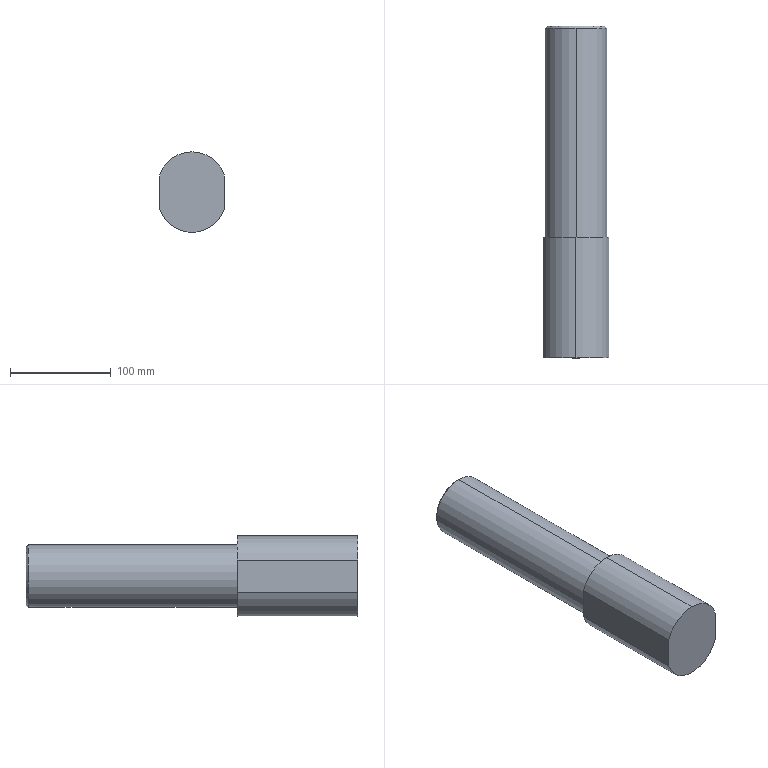Part | SolidWorks | features MirrorStock 1 | 1 solid | 16 faces | box 65 x 330 x 80 mm | volume 1156605 mm3 | cylinder 7 | plane 5 | cone 4 | commonest cylinder face diameters 68 x3 8.5 x2 62 x2
STEP:
#1=CARTESIAN_POINT('',(0.,330.,29.));
#2=VERTEX_POINT('',#1);
#3=CARTESIAN_POINT('',(0.,330.,-29.));
#4=VERTEX_POINT('',#3);
#5=CARTESIAN_POINT('',(0.,330.,0.));
#6=DIRECTION('',(0.,-1.,0.));
#7=DIRECTION('',(0.,0.,-1.));
#8=AXIS2_PLACEMENT_3D('',#5,#6,#7);
#9=CIRCLE('',#8,29.);
#10=EDGE_CURVE('',#2,#4,#9,.T.);
#11=ORIENTED_EDGE('',*,*,#10,.T.);
#12=CARTESIAN_POINT('',(0.,328.,-31.));
#13=VERTEX_POINT('',#12);
#14=CARTESIAN_POINT('',(0.,330.,-29.));
#15=DIRECTION('',(0.,-0.7071,-0.7071));
#16=VECTOR('',#15,1000.);
#17=LINE('',#14,#16);
#18=EDGE_CURVE('',#4,#13,#17,.T.);
#19=ORIENTED_EDGE('',*,*,#18,.T.);
#20=CARTESIAN_POINT('',(0.,328.,31.));
#21=VERTEX_POINT('',#20);
#22=CARTESIAN_POINT('',(0.,328.,0.));
#23=DIRECTION('',(0.,1.,0.));
#24=DIRECTION('',(0.,0.,-1.));
#25=AXIS2_PLACEMENT_3D('',#22,#23,#24);
#26=CIRCLE('',#25,31.);
#27=EDGE_CURVE('',#13,#21,#26,.T.);
#28=ORIENTED_EDGE('',*,*,#27,.T.);
#29=CARTESIAN_POINT('',(0.,330.,29.));
#30=DIRECTION('',(0.,-0.7071,0.7071));
#31=VECTOR('',#30,1000.);
#32=LINE('',#29,#31);
#33=EDGE_CURVE('',#2,#21,#32,.T.);
#34=ORIENTED_EDGE('',*,*,#33,.F.);
#35=EDGE_LOOP('',(#11,#19,#28,#34));
#36=FACE_OUTER_BOUND('',#35,.T.);
#37=CARTESIAN_POINT('',(0.,330.,0.));
#38=DIRECTION('',(0.,-1.,0.));
#39=DIRECTION('',(0.,0.,1.));
#40=AXIS2_PLACEMENT_3D('',#37,#38,#39);
#41=CONICAL_SURFACE('',#40,29.,0.7854);
#42=ADVANCED_FACE('',(#36),#41,.T.);
#43=CARTESIAN_POINT('',(0.,285.,-0.9463));
#44=VERTEX_POINT('',#43);
#45=CARTESIAN_POINT('',(4.25,285.,-3.5));
#46=VERTEX_POINT('',#45);
#47=CARTESIAN_POINT('',(4.25,285.,-3.5));
#48=DIRECTION('',(0.8572,0.,-0.515));
#49=VECTOR('',#48,1000.);
#50=LINE('',#47,#49);
#51=EDGE_CURVE('',#44,#46,#50,.T.);
#52=ORIENTED_EDGE('',*,*,#51,.F.);
#53=CARTESIAN_POINT('',(-4.25,285.,-3.5));
#54=VERTEX_POINT('',#53);
#55=CARTESIAN_POINT('',(-4.25,285.,-3.5));
#56=DIRECTION('',(-0.8572,0.,-0.515));
#57=VECTOR('',#56,1000.);
#58=LINE('',#55,#57);
#59=EDGE_CURVE('',#44,#54,#58,.T.);
#60=ORIENTED_EDGE('',*,*,#59,.T.);
#61=CARTESIAN_POINT('',(0.,285.,-3.5));
#62=DIRECTION('',(0.,0.,1.));
#63=DIRECTION('',(1.,0.,0.));
#64=AXIS2_PLACEMENT_3D('',#61,#62,#63);
#65=CIRCLE('',#64,4.25);
#66=EDGE_CURVE('',#46,#54,#65,.T.);
#67=ORIENTED_EDGE('',*,*,#66,.F.);
#68=EDGE_LOOP('',(#52,#60,#67));
#69=FACE_OUTER_BOUND('',#68,.T.);
#70=CARTESIAN_POINT('',(0.,285.,-3.5));
#71=DIRECTION('',(0.,0.,-1.));
#72=DIRECTION('',(1.,0.,0.));
#73=AXIS2_PLACEMENT_3D('',#70,#71,#72);
#74=CONICAL_SURFACE('',#73,4.25,1.03);
#75=ADVANCED_FACE('',(#69),#74,.F.);
#76=ORIENTED_EDGE('',*,*,#66,.T.);
#77=CARTESIAN_POINT('',(-4.25,285.,-30.707));
#78=VERTEX_POINT('',#77);
#79=CARTESIAN_POINT('',(-4.25,285.,-31.));
#80=DIRECTION('',(0.,0.,-1.));
#81=VECTOR('',#80,1000.);
#82=LINE('',#79,#81);
#83=EDGE_CURVE('',#54,#78,#82,.T.);
#84=ORIENTED_EDGE('',*,*,#83,.T.);
#85=CARTESIAN_POINT('',(0.,289.25,-31.));
#86=VERTEX_POINT('',#85);
#87=CARTESIAN_POINT('',(-4.25,285.,-30.707));
#88=CARTESIAN_POINT('',(-4.25,285.278,-30.707));
#89=CARTESIAN_POINT('',(-4.223,285.554,-30.711));
#90=CARTESIAN_POINT('',(-4.114,286.103,-30.726));
#91=CARTESIAN_POINT('',(-4.032,286.371,-30.737));
#92=CARTESIAN_POINT('',(-3.82,286.883,-30.764));
#93=CARTESIAN_POINT('',(-3.688,287.13,-30.78));
#94=CARTESIAN_POINT('',(-3.378,287.594,-30.816));
#95=CARTESIAN_POINT('',(-3.202,287.808,-30.835));
#96=CARTESIAN_POINT('',(-2.81,288.2,-30.873));
#97=CARTESIAN_POINT('',(-2.592,288.38,-30.892));
#98=CARTESIAN_POINT('',(-2.13,288.688,-30.928));
#99=CARTESIAN_POINT('',(-1.886,288.819,-30.944));
#100=CARTESIAN_POINT('',(-1.371,289.032,-30.971));
#101=CARTESIAN_POINT('',(-1.102,289.114,-30.982));
#102=CARTESIAN_POINT('',(-0.5579,289.222,-30.996));
#103=CARTESIAN_POINT('',(-0.281,289.25,-31.));
#104=CARTESIAN_POINT('',(0.,289.25,-31.));
#105=B_SPLINE_CURVE_WITH_KNOTS('',3,(#87,#88,#89,#90,#91,#92,#93,#94,#95,#96,#97,#98,#99,#100,#101,#102,#103,#104),.UNSPECIFIED.,.F.,.F.,(4,2,2,2,2,2,2,2,4),(0.0133,0.01413,0.01497,0.0158,0.01663,0.01746,0.01829,0.01912,0.01996),.UNSPECIFIED.);
#106=EDGE_CURVE('',#78,#86,#105,.T.);
#107=ORIENTED_EDGE('',*,*,#106,.T.);
#108=CARTESIAN_POINT('',(4.25,285.,-30.707));
#109=VERTEX_POINT('',#108);
#110=CARTESIAN_POINT('',(0.,289.25,-31.));
#111=CARTESIAN_POINT('',(0.2808,289.25,-31.));
#112=CARTESIAN_POINT('',(0.5569,289.222,-30.996));
#113=CARTESIAN_POINT('',(1.1,289.114,-30.982));
#114=CARTESIAN_POINT('',(1.371,289.033,-30.971));
#115=CARTESIAN_POINT('',(1.885,288.819,-30.944));
#116=CARTESIAN_POINT('',(2.128,288.689,-30.928));
#117=CARTESIAN_POINT('',(2.59,288.381,-30.892));
#118=CARTESIAN_POINT('',(2.808,288.202,-30.873));
#119=CARTESIAN_POINT('',(3.2,287.811,-30.835));
#120=CARTESIAN_POINT('',(3.376,287.597,-30.816));
#121=CARTESIAN_POINT('',(3.687,287.133,-30.78));
#122=CARTESIAN_POINT('',(3.818,286.886,-30.764));
#123=CARTESIAN_POINT('',(4.031,286.376,-30.737));
#124=CARTESIAN_POINT('',(4.113,286.108,-30.726));
#125=CARTESIAN_POINT('',(4.222,285.559,-30.711));
#126=CARTESIAN_POINT('',(4.25,285.281,-30.707));
#127=CARTESIAN_POINT('',(4.25,285.,-30.707));
#128=B_SPLINE_CURVE_WITH_KNOTS('',3,(#110,#111,#112,#113,#114,#115,#116,#117,#118,#119,#120,#121,#122,#123,#124,#125,#126,#127),.UNSPECIFIED.,.F.,.F.,(4,2,2,2,2,2,2,2,4),(0.01996,0.02079,0.02162,0.02245,0.02328,0.02411,0.02494,0.02577,0.0266),.UNSPECIFIED.);
#129=EDGE_CURVE('',#86,#109,#128,.T.);
#130=ORIENTED_EDGE('',*,*,#129,.T.);
#131=CARTESIAN_POINT('',(4.25,285.,-31.));
#132=DIRECTION('',(0.,0.,-1.));
#133=VECTOR('',#132,1000.);
#134=LINE('',#131,#133);
#135=EDGE_CURVE('',#46,#109,#134,.T.);
#136=ORIENTED_EDGE('',*,*,#135,.F.);
#137=EDGE_LOOP('',(#76,#84,#107,#130,#136));
#138=FACE_OUTER_BOUND('',#137,.T.);
#139=CARTESIAN_POINT('',(0.,285.,-31.));
#140=DIRECTION('',(0.,0.,-1.));
#141=DIRECTION('',(1.,0.,0.));
#142=AXIS2_PLACEMENT_3D('',#139,#140,#141);
#143=CYLINDRICAL_SURFACE('',#142,4.25);
#144=ADVANCED_FACE('',(#138),#143,.F.);
#145=ORIENTED_EDGE('',*,*,#27,.F.);
#146=CARTESIAN_POINT('',(0.,330.,-31.));
#147=DIRECTION('',(0.,-1.,0.));
#148=VECTOR('',#147,1000.);
#149=LINE('',#146,#148);
#150=EDGE_CURVE('',#13,#86,#149,.T.);
#151=ORIENTED_EDGE('',*,*,#150,.T.);
#152=ORIENTED_EDGE('',*,*,#106,.F.);
#153=CARTESIAN_POINT('',(0.,280.75,-31.));
#154=VERTEX_POINT('',#153);
#155=CARTESIAN_POINT('',(0.,280.75,-31.));
#156=CARTESIAN_POINT('',(-0.2775,280.75,-31.));
#157=CARTESIAN_POINT('',(-0.5594,280.778,-30.996));
#158=CARTESIAN_POINT('',(-1.105,280.887,-30.982));
#159=CARTESIAN_POINT('',(-1.37,280.967,-30.971));
#160=CARTESIAN_POINT('',(-1.884,281.18,-30.944));
#161=CARTESIAN_POINT('',(-2.133,281.313,-30.927));
#162=CARTESIAN_POINT('',(-2.593,281.621,-30.892));
#163=CARTESIAN_POINT('',(-2.807,281.797,-30.873));
#164=CARTESIAN_POINT('',(-3.204,282.193,-30.835));
#165=CARTESIAN_POINT('',(-3.379,282.408,-30.816));
#166=CARTESIAN_POINT('',(-3.687,282.868,-30.78));
#167=CARTESIAN_POINT('',(-3.82,283.116,-30.764));
#168=CARTESIAN_POINT('',(-4.033,283.631,-30.737));
#169=CARTESIAN_POINT('',(-4.113,283.895,-30.726));
#170=CARTESIAN_POINT('',(-4.222,284.441,-30.711));
#171=CARTESIAN_POINT('',(-4.25,284.723,-30.707));
#172=CARTESIAN_POINT('',(-4.25,285.,-30.707));
#173=B_SPLINE_CURVE_WITH_KNOTS('',3,(#155,#156,#157,#158,#159,#160,#161,#162,#163,#164,#165,#166,#167,#168,#169,#170,#171,#172),.UNSPECIFIED.,.F.,.F.,(4,2,2,2,2,2,2,2,4),(0.006653,0.007484,0.008316,0.009147,0.009978,0.01081,0.01164,0.01247,0.0133),.UNSPECIFIED.);
#174=EDGE_CURVE('',#154,#78,#173,.T.);
#175=ORIENTED_EDGE('',*,*,#174,.F.);
#176=CARTESIAN_POINT('',(0.,120.,-31.));
#177=VERTEX_POINT('',#176);
#178=CARTESIAN_POINT('',(0.,330.,-31.));
#179=DIRECTION('',(0.,-1.,0.));
#180=VECTOR('',#179,1000.);
#181=LINE('',#178,#180);
#182=EDGE_CURVE('',#154,#177,#181,.T.);
#183=ORIENTED_EDGE('',*,*,#182,.T.);
#184=CARTESIAN_POINT('',(0.,120.,31.));
#185=VERTEX_POINT('',#184);
#186=CARTESIAN_POINT('',(0.,120.,0.));
#187=DIRECTION('',(0.,-1.,0.));
#188=DIRECTION('',(0.,0.,-1.));
#189=AXIS2_PLACEMENT_3D('',#186,#187,#188);
#190=CIRCLE('',#189,31.);
#191=EDGE_CURVE('',#185,#177,#190,.T.);
#192=ORIENTED_EDGE('',*,*,#191,.F.);
#193=CARTESIAN_POINT('',(0.,330.,31.));
#194=DIRECTION('',(0.,-1.,0.));
#195=VECTOR('',#194,1000.);
#196=LINE('',#193,#195);
#197=EDGE_CURVE('',#21,#185,#196,.T.);
#198=ORIENTED_EDGE('',*,*,#197,.F.);
#199=EDGE_LOOP('',(#145,#151,#152,#175,#183,#192,#198));
#200=FACE_OUTER_BOUND('',#199,.T.);
#201=CARTESIAN_POINT('',(0.,330.,0.));
#202=DIRECTION('',(0.,-1.,0.));
#203=DIRECTION('',(0.,0.,1.));
#204=AXIS2_PLACEMENT_3D('',#201,#202,#203);
#205=CYLINDRICAL_SURFACE('',#204,31.);
#206=ADVANCED_FACE('',(#200),#205,.T.);
#207=CARTESIAN_POINT('',(32.5,120.,15.987));
#208=VERTEX_POINT('',#207);
#209=CARTESIAN_POINT('',(0.,120.,40.));
#210=VERTEX_POINT('',#209);
#211=CARTESIAN_POINT('',(0.,120.,6.));
#212=DIRECTION('',(0.,-1.,0.));
#213=DIRECTION('',(0.,0.,-1.));
#214=AXIS2_PLACEMENT_3D('',#211,#212,#213);
#215=CIRCLE('',#214,34.);
#216=EDGE_CURVE('',#208,#210,#215,.T.);
#217=ORIENTED_EDGE('',*,*,#216,.T.);
#218=CARTESIAN_POINT('',(0.,0.,40.));
#219=VERTEX_POINT('',#218);
#220=CARTESIAN_POINT('',(0.,120.,40.));
#221=DIRECTION('',(0.,-1.,0.));
#222=VECTOR('',#221,1000.);
#223=LINE('',#220,#222);
#224=EDGE_CURVE('',#210,#219,#223,.T.);
#225=ORIENTED_EDGE('',*,*,#224,.T.);
#226=CARTESIAN_POINT('',(32.5,0.,15.987));
#227=VERTEX_POINT('',#226);
#228=CARTESIAN_POINT('',(0.,0.,6.));
#229=DIRECTION('',(0.,-1.,0.));
#230=DIRECTION('',(0.,0.,-1.));
#231=AXIS2_PLACEMENT_3D('',#228,#229,#230);
#232=CIRCLE('',#231,34.);
#233=EDGE_CURVE('',#227,#219,#232,.T.);
#234=ORIENTED_EDGE('',*,*,#233,.F.);
#235=CARTESIAN_POINT('',(32.5,120.,15.987));
#236=DIRECTION('',(0.,-1.,0.));
#237=VECTOR('',#236,1000.);
#238=LINE('',#235,#237);
#239=EDGE_CURVE('',#208,#227,#238,.T.);
#240=ORIENTED_EDGE('',*,*,#239,.F.);
#241=EDGE_LOOP('',(#217,#225,#234,#240));
#242=FACE_OUTER_BOUND('',#241,.T.);
#243=CARTESIAN_POINT('',(0.,120.,6.));
#244=DIRECTION('',(0.,-1.,0.));
#245=DIRECTION('',(0.,0.,1.));
#246=AXIS2_PLACEMENT_3D('',#243,#244,#245);
#247=CYLINDRICAL_SURFACE('',#246,34.);
#248=ADVANCED_FACE('',(#242),#247,.T.);
#249=ORIENTED_EDGE('',*,*,#224,.F.);
#250=CARTESIAN_POINT('',(-32.5,120.,15.987));
#251=VERTEX_POINT('',#250);
#252=CARTESIAN_POINT('',(0.,120.,6.));
#253=DIRECTION('',(0.,-1.,0.));
#254=DIRECTION('',(0.,0.,-1.));
#255=AXIS2_PLACEMENT_3D('',#252,#253,#254);
#256=CIRCLE('',#255,34.);
#257=EDGE_CURVE('',#210,#251,#256,.T.);
#258=ORIENTED_EDGE('',*,*,#257,.T.);
#259=CARTESIAN_POINT('',(-32.5,0.,15.987));
#260=VERTEX_POINT('',#259);
#261=CARTESIAN_POINT('',(-32.5,120.,15.987));
#262=DIRECTION('',(0.,-1.,0.));
#263=VECTOR('',#262,1000.);
#264=LINE('',#261,#263);
#265=EDGE_CURVE('',#251,#260,#264,.T.);
#266=ORIENTED_EDGE('',*,*,#265,.T.);
#267=CARTESIAN_POINT('',(0.,0.,6.));
#268=DIRECTION('',(0.,-1.,0.));
#269=DIRECTION('',(0.,0.,-1.));
#270=AXIS2_PLACEMENT_3D('',#267,#268,#269);
#271=CIRCLE('',#270,34.);
#272=EDGE_CURVE('',#219,#260,#271,.T.);
#273=ORIENTED_EDGE('',*,*,#272,.F.);
#274=EDGE_LOOP('',(#249,#258,#266,#273));
#275=FACE_OUTER_BOUND('',#274,.T.);
#276=CARTESIAN_POINT('',(0.,120.,6.));
#277=DIRECTION('',(0.,-1.,0.));
#278=DIRECTION('',(0.,0.,1.));
#279=AXIS2_PLACEMENT_3D('',#276,#277,#278);
#280=CYLINDRICAL_SURFACE('',#279,34.);
#281=ADVANCED_FACE('',(#275),#280,.T.);
#282=CARTESIAN_POINT('',(-32.5,0.,-15.987));
#283=VERTEX_POINT('',#282);
#284=CARTESIAN_POINT('',(-32.5,0.,-15.987));
#285=DIRECTION('',(0.,0.,-1.));
#286=VECTOR('',#285,1000.);
#287=LINE('',#284,#286);
#288=EDGE_CURVE('',#260,#283,#287,.T.);
#289=ORIENTED_EDGE('',*,*,#288,.F.);
#290=ORIENTED_EDGE('',*,*,#265,.F.);
#291=CARTESIAN_POINT('',(-32.5,120.,-15.987));
#292=VERTEX_POINT('',#291);
#293=CARTESIAN_POINT('',(-32.5,120.,-15.987));
#294=DIRECTION('',(0.,0.,-1.));
#295=VECTOR('',#294,1000.);
#296=LINE('',#293,#295);
#297=EDGE_CURVE('',#251,#292,#296,.T.);
#298=ORIENTED_EDGE('',*,*,#297,.T.);
#299=CARTESIAN_POINT('',(-32.5,120.,-15.987));
#300=DIRECTION('',(0.,-1.,0.));
#301=VECTOR('',#300,1000.);
#302=LINE('',#299,#301);
#303=EDGE_CURVE('',#292,#283,#302,.T.);
#304=ORIENTED_EDGE('',*,*,#303,.T.);
#305=EDGE_LOOP('',(#289,#290,#298,#304));
#306=FACE_OUTER_BOUND('',#305,.T.);
#307=CARTESIAN_POINT('',(-32.5,120.,-15.987));
#308=DIRECTION('',(1.,0.,0.));
#309=DIRECTION('',(0.,0.,1.));
#310=AXIS2_PLACEMENT_3D('',#307,#308,#309);
#311=PLANE('',#310);
#312=ADVANCED_FACE('',(#306),#311,.F.);
#313=CARTESIAN_POINT('',(32.5,0.,-15.987));
#314=VERTEX_POINT('',#313);
#315=CARTESIAN_POINT('',(0.,0.,-6.));
#316=DIRECTION('',(0.,-1.,0.));
#317=DIRECTION('',(0.,0.,1.));
#318=AXIS2_PLACEMENT_3D('',#315,#316,#317);
#319=CIRCLE('',#318,34.);
#320=EDGE_CURVE('',#283,#314,#319,.T.);
#321=ORIENTED_EDGE('',*,*,#320,.F.);
#322=ORIENTED_EDGE('',*,*,#303,.F.);
#323=CARTESIAN_POINT('',(32.5,120.,-15.987));
#324=VERTEX_POINT('',#323);
#325=CARTESIAN_POINT('',(0.,120.,-6.));
#326=DIRECTION('',(0.,-1.,0.));
#327=DIRECTION('',(0.,0.,1.));
#328=AXIS2_PLACEMENT_3D('',#325,#326,#327);
#329=CIRCLE('',#328,34.);
#330=EDGE_CURVE('',#292,#324,#329,.T.);
#331=ORIENTED_EDGE('',*,*,#330,.T.);
#332=CARTESIAN_POINT('',(32.5,120.,-15.987));
#333=DIRECTION('',(0.,-1.,0.));
#334=VECTOR('',#333,1000.);
#335=LINE('',#332,#334);
#336=EDGE_CURVE('',#324,#314,#335,.T.);
#337=ORIENTED_EDGE('',*,*,#336,.T.);
#338=EDGE_LOOP('',(#321,#322,#331,#337));
#339=FACE_OUTER_BOUND('',#338,.T.);
#340=CARTESIAN_POINT('',(0.,120.,-6.));
#341=DIRECTION('',(0.,-1.,0.));
#342=DIRECTION('',(0.,0.,1.));
#343=AXIS2_PLACEMENT_3D('',#340,#341,#342);
#344=CYLINDRICAL_SURFACE('',#343,34.);
#345=ADVANCED_FACE('',(#339),#344,.T.);
#346=CARTESIAN_POINT('',(32.5,0.,-15.987));
#347=DIRECTION('',(0.,0.,1.));
#348=VECTOR('',#347,1000.);
#349=LINE('',#346,#348);
#350=EDGE_CURVE('',#314,#227,#349,.T.);
#351=ORIENTED_EDGE('',*,*,#350,.F.);
#352=ORIENTED_EDGE('',*,*,#336,.F.);
#353=CARTESIAN_POINT('',(32.5,120.,-15.987));
#354=DIRECTION('',(0.,0.,1.));
#355=VECTOR('',#354,1000.);
#356=LINE('',#353,#355);
#357=EDGE_CURVE('',#324,#208,#356,.T.);
#358=ORIENTED_EDGE('',*,*,#357,.T.);
#359=ORIENTED_EDGE('',*,*,#239,.T.);
#360=EDGE_LOOP('',(#351,#352,#358,#359));
#361=FACE_OUTER_BOUND('',#360,.T.);
#362=CARTESIAN_POINT('',(32.5,120.,-15.987));
#363=DIRECTION('',(-1.,0.,0.));
#364=DIRECTION('',(0.,0.,-1.));
#365=AXIS2_PLACEMENT_3D('',#362,#363,#364);
#366=PLANE('',#365);
#367=ADVANCED_FACE('',(#361),#366,.F.);
#368=ORIENTED_EDGE('',*,*,#191,.T.);
#369=CARTESIAN_POINT('',(0.,120.,0.));
#370=DIRECTION('',(0.,-1.,0.));
#371=DIRECTION('',(0.,0.,-1.));
#372=AXIS2_PLACEMENT_3D('',#369,#370,#371);
#373=CIRCLE('',#372,31.);
#374=EDGE_CURVE('',#177,#185,#373,.T.);
#375=ORIENTED_EDGE('',*,*,#374,.T.);
#376=EDGE_LOOP('',(#368,#375));
#377=FACE_BOUND('',#376,.T.);
#378=ORIENTED_EDGE('',*,*,#216,.F.);
#379=ORIENTED_EDGE('',*,*,#357,.F.);
#380=ORIENTED_EDGE('',*,*,#330,.F.);
#381=ORIENTED_EDGE('',*,*,#297,.F.);
#382=ORIENTED_EDGE('',*,*,#257,.F.);
#383=EDGE_LOOP('',(#378,#379,#380,#381,#382));
#384=FACE_OUTER_BOUND('',#383,.T.);
#385=CARTESIAN_POINT('',(0.,120.,6.));
#386=DIRECTION('',(0.,1.,0.));
#387=DIRECTION('',(0.,0.,-1.));
#388=AXIS2_PLACEMENT_3D('',#385,#386,#387);
#389=PLANE('',#388);
#390=ADVANCED_FACE('',(#377,#384),#389,.T.);
#391=ORIENTED_EDGE('',*,*,#233,.T.);
#392=ORIENTED_EDGE('',*,*,#272,.T.);
#393=ORIENTED_EDGE('',*,*,#288,.T.);
#394=ORIENTED_EDGE('',*,*,#320,.T.);
#395=ORIENTED_EDGE('',*,*,#350,.T.);
#396=EDGE_LOOP('',(#391,#392,#393,#394,#395));
#397=FACE_OUTER_BOUND('',#396,.T.);
#398=CARTESIAN_POINT('',(0.,0.,6.));
#399=DIRECTION('',(0.,1.,0.));
#400=DIRECTION('',(0.,0.,-1.));
#401=AXIS2_PLACEMENT_3D('',#398,#399,#400);
#402=PLANE('',#401);
#403=ADVANCED_FACE('',(#397),#402,.F.);
#404=ORIENTED_EDGE('',*,*,#150,.F.);
#405=CARTESIAN_POINT('',(0.,328.,0.));
#406=DIRECTION('',(0.,1.,0.));
#407=DIRECTION('',(0.,0.,-1.));
#408=AXIS2_PLACEMENT_3D('',#405,#406,#407);
#409=CIRCLE('',#408,31.);
#410=EDGE_CURVE('',#21,#13,#409,.T.);
#411=ORIENTED_EDGE('',*,*,#410,.F.);
#412=ORIENTED_EDGE('',*,*,#197,.T.);
#413=ORIENTED_EDGE('',*,*,#374,.F.);
#414=ORIENTED_EDGE('',*,*,#182,.F.);
#415=CARTESIAN_POINT('',(4.25,285.,-30.707));
#416=CARTESIAN_POINT('',(4.25,284.719,-30.707));
#417=CARTESIAN_POINT('',(4.222,284.442,-30.711));
#418=CARTESIAN_POINT('',(4.114,283.899,-30.726));
#419=CARTESIAN_POINT('',(4.032,283.628,-30.737));
#420=CARTESIAN_POINT('',(3.819,283.114,-30.764));
#421=CARTESIAN_POINT('',(3.688,282.87,-30.78));
#422=CARTESIAN_POINT('',(3.379,282.408,-30.816));
#423=CARTESIAN_POINT('',(3.2,282.189,-30.835));
#424=CARTESIAN_POINT('',(2.808,281.798,-30.873));
#425=CARTESIAN_POINT('',(2.594,281.622,-30.892));
#426=CARTESIAN_POINT('',(2.13,281.311,-30.928));
#427=CARTESIAN_POINT('',(1.883,281.18,-30.944));
#428=CARTESIAN_POINT('',(1.371,280.968,-30.971));
#429=CARTESIAN_POINT('',(1.103,280.886,-30.982));
#430=CARTESIAN_POINT('',(0.5537,280.777,-30.996));
#431=CARTESIAN_POINT('',(0.2776,280.75,-31.));
#432=CARTESIAN_POINT('',(0.,280.75,-31.));
#433=B_SPLINE_CURVE_WITH_KNOTS('',3,(#415,#416,#417,#418,#419,#420,#421,#422,#423,#424,#425,#426,#427,#428,#429,#430,#431,#432),.UNSPECIFIED.,.F.,.F.,(4,2,2,2,2,2,2,2,4),(0.,0.0008316,0.001663,0.002495,0.003327,0.004158,0.00499,0.005821,0.006653),.UNSPECIFIED.);
#434=EDGE_CURVE('',#109,#154,#433,.T.);
#435=ORIENTED_EDGE('',*,*,#434,.F.);
#436=ORIENTED_EDGE('',*,*,#129,.F.);
#437=EDGE_LOOP('',(#404,#411,#412,#413,#414,#435,#436));
#438=FACE_OUTER_BOUND('',#437,.T.);
#439=CARTESIAN_POINT('',(0.,330.,0.));
#440=DIRECTION('',(0.,-1.,0.));
#441=DIRECTION('',(0.,0.,1.));
#442=AXIS2_PLACEMENT_3D('',#439,#440,#441);
#443=CYLINDRICAL_SURFACE('',#442,31.);
#444=ADVANCED_FACE('',(#438),#443,.T.);
#445=ORIENTED_EDGE('',*,*,#10,.F.);
#446=CARTESIAN_POINT('',(0.,330.,0.));
#447=DIRECTION('',(0.,-1.,0.));
#448=DIRECTION('',(0.,0.,-1.));
#449=AXIS2_PLACEMENT_3D('',#446,#447,#448);
#450=CIRCLE('',#449,29.);
#451=EDGE_CURVE('',#4,#2,#450,.T.);
#452=ORIENTED_EDGE('',*,*,#451,.F.);
#453=EDGE_LOOP('',(#445,#452));
#454=FACE_OUTER_BOUND('',#453,.T.);
#455=CARTESIAN_POINT('',(0.,330.,0.));
#456=DIRECTION('',(0.,1.,0.));
#457=DIRECTION('',(0.,0.,-1.));
#458=AXIS2_PLACEMENT_3D('',#455,#456,#457);
#459=PLANE('',#458);
#460=ADVANCED_FACE('',(#454),#459,.T.);
#461=ORIENTED_EDGE('',*,*,#83,.F.);
#462=CARTESIAN_POINT('',(0.,285.,-3.5));
#463=DIRECTION('',(0.,0.,1.));
#464=DIRECTION('',(1.,0.,0.));
#465=AXIS2_PLACEMENT_3D('',#462,#463,#464);
#466=CIRCLE('',#465,4.25);
#467=EDGE_CURVE('',#54,#46,#466,.T.);
#468=ORIENTED_EDGE('',*,*,#467,.T.);
#469=ORIENTED_EDGE('',*,*,#135,.T.);
#470=ORIENTED_EDGE('',*,*,#434,.T.);
#471=ORIENTED_EDGE('',*,*,#174,.T.);
#472=EDGE_LOOP('',(#461,#468,#469,#470,#471));
#473=FACE_OUTER_BOUND('',#472,.T.);
#474=CARTESIAN_POINT('',(0.,285.,-31.));
#475=DIRECTION('',(0.,0.,-1.));
#476=DIRECTION('',(1.,0.,0.));
#477=AXIS2_PLACEMENT_3D('',#474,#475,#476);
#478=CYLINDRICAL_SURFACE('',#477,4.25);
#479=ADVANCED_FACE('',(#473),#478,.F.);
#480=ORIENTED_EDGE('',*,*,#59,.F.);
#481=ORIENTED_EDGE('',*,*,#51,.T.);
#482=ORIENTED_EDGE('',*,*,#467,.F.);
#483=EDGE_LOOP('',(#480,#481,#482));
#484=FACE_OUTER_BOUND('',#483,.T.);
#485=CARTESIAN_POINT('',(0.,285.,-3.5));
#486=DIRECTION('',(0.,0.,-1.));
#487=DIRECTION('',(1.,0.,0.));
#488=AXIS2_PLACEMENT_3D('',#485,#486,#487);
#489=CONICAL_SURFACE('',#488,4.25,1.03);
#490=ADVANCED_FACE('',(#484),#489,.F.);
#491=ORIENTED_EDGE('',*,*,#18,.F.);
#492=ORIENTED_EDGE('',*,*,#451,.T.);
#493=ORIENTED_EDGE('',*,*,#33,.T.);
#494=ORIENTED_EDGE('',*,*,#410,.T.);
#495=EDGE_LOOP('',(#491,#492,#493,#494));
#496=FACE_OUTER_BOUND('',#495,.T.);
#497=CARTESIAN_POINT('',(0.,330.,0.));
#498=DIRECTION('',(0.,-1.,0.));
#499=DIRECTION('',(0.,0.,1.));
#500=AXIS2_PLACEMENT_3D('',#497,#498,#499);
#501=CONICAL_SURFACE('',#500,29.,0.7854);
#502=ADVANCED_FACE('',(#496),#501,.T.);
#503=CLOSED_SHELL('',(#42,#75,#144,#206,#248,#281,#312,#345,#367,#390,#403,#444,#460,#479,#490,#502));
#504=MANIFOLD_SOLID_BREP('',#503);
#505=CARTESIAN_POINT('',(0.,0.,0.));
#506=DIRECTION('',(0.,0.,1.));
#507=DIRECTION('',(1.,0.,0.));
#508=AXIS2_PLACEMENT_3D('',#505,#506,#507);
#509=(LENGTH_UNIT()NAMED_UNIT(*)SI_UNIT(.MILLI.,.METRE.));
#510=UNCERTAINTY_MEASURE_WITH_UNIT(LENGTH_MEASURE(0.00001),#509,'','');
#511=(NAMED_UNIT(*)PLANE_ANGLE_UNIT()SI_UNIT($,.RADIAN.));
#512=(NAMED_UNIT(*)SI_UNIT($,.STERADIAN.)SOLID_ANGLE_UNIT());
#513=(GEOMETRIC_REPRESENTATION_CONTEXT(3)GLOBAL_UNCERTAINTY_ASSIGNED_CONTEXT((#510))GLOBAL_UNIT_ASSIGNED_CONTEXT((#509,#511,#512))REPRESENTATION_CONTEXT('',''));
#514=ADVANCED_BREP_SHAPE_REPRESENTATION('',(#504,#508),#513);